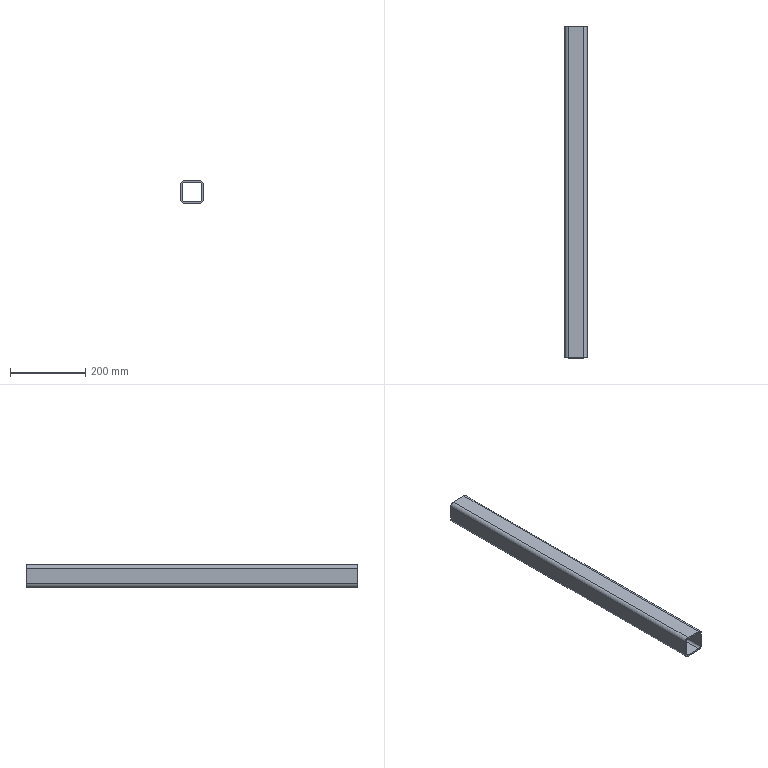Part | SolidWorks | features Extrusion 1 | 1 solid | 18 faces | box 60 x 880 x 60 mm | volume 740134 mm3 | plane 10 | cylinder 8 | commonest cylinder face diameters 12 x4 20 x4
STEP:
#1=CARTESIAN_POINT('',(20.,880.,30.));
#2=VERTEX_POINT('',#1);
#3=CARTESIAN_POINT('',(30.,880.,20.));
#4=VERTEX_POINT('',#3);
#5=CARTESIAN_POINT('',(20.,880.,20.));
#6=DIRECTION('',(0.,1.,0.));
#7=DIRECTION('',(0.,0.,1.));
#8=AXIS2_PLACEMENT_3D('',#5,#6,#7);
#9=CIRCLE('',#8,10.);
#10=EDGE_CURVE('',#2,#4,#9,.T.);
#11=ORIENTED_EDGE('',*,*,#10,.T.);
#12=CARTESIAN_POINT('',(30.,880.,-20.));
#13=VERTEX_POINT('',#12);
#14=CARTESIAN_POINT('',(30.,880.,20.));
#15=DIRECTION('',(0.,0.,-1.));
#16=VECTOR('',#15,1000.);
#17=LINE('',#14,#16);
#18=EDGE_CURVE('',#4,#13,#17,.T.);
#19=ORIENTED_EDGE('',*,*,#18,.T.);
#20=CARTESIAN_POINT('',(20.,880.,-30.));
#21=VERTEX_POINT('',#20);
#22=CARTESIAN_POINT('',(20.,880.,-20.));
#23=DIRECTION('',(0.,1.,0.));
#24=DIRECTION('',(0.,0.,-1.));
#25=AXIS2_PLACEMENT_3D('',#22,#23,#24);
#26=CIRCLE('',#25,10.);
#27=EDGE_CURVE('',#13,#21,#26,.T.);
#28=ORIENTED_EDGE('',*,*,#27,.T.);
#29=CARTESIAN_POINT('',(-20.,880.,-30.));
#30=VERTEX_POINT('',#29);
#31=CARTESIAN_POINT('',(-20.,880.,-30.));
#32=DIRECTION('',(-1.,0.,0.));
#33=VECTOR('',#32,1000.);
#34=LINE('',#31,#33);
#35=EDGE_CURVE('',#21,#30,#34,.T.);
#36=ORIENTED_EDGE('',*,*,#35,.T.);
#37=CARTESIAN_POINT('',(-30.,880.,-20.));
#38=VERTEX_POINT('',#37);
#39=CARTESIAN_POINT('',(-20.,880.,-20.));
#40=DIRECTION('',(0.,1.,0.));
#41=DIRECTION('',(0.,0.,-1.));
#42=AXIS2_PLACEMENT_3D('',#39,#40,#41);
#43=CIRCLE('',#42,10.);
#44=EDGE_CURVE('',#30,#38,#43,.T.);
#45=ORIENTED_EDGE('',*,*,#44,.T.);
#46=CARTESIAN_POINT('',(-30.,880.,20.));
#47=VERTEX_POINT('',#46);
#48=CARTESIAN_POINT('',(-30.,880.,20.));
#49=DIRECTION('',(0.,0.,1.));
#50=VECTOR('',#49,1000.);
#51=LINE('',#48,#50);
#52=EDGE_CURVE('',#38,#47,#51,.T.);
#53=ORIENTED_EDGE('',*,*,#52,.T.);
#54=CARTESIAN_POINT('',(-20.,880.,30.));
#55=VERTEX_POINT('',#54);
#56=CARTESIAN_POINT('',(-20.,880.,20.));
#57=DIRECTION('',(0.,1.,0.));
#58=DIRECTION('',(0.,0.,-1.));
#59=AXIS2_PLACEMENT_3D('',#56,#57,#58);
#60=CIRCLE('',#59,10.);
#61=EDGE_CURVE('',#47,#55,#60,.T.);
#62=ORIENTED_EDGE('',*,*,#61,.T.);
#63=CARTESIAN_POINT('',(-20.,880.,30.));
#64=DIRECTION('',(1.,0.,0.));
#65=VECTOR('',#64,1000.);
#66=LINE('',#63,#65);
#67=EDGE_CURVE('',#55,#2,#66,.T.);
#68=ORIENTED_EDGE('',*,*,#67,.T.);
#69=EDGE_LOOP('',(#11,#19,#28,#36,#45,#53,#62,#68));
#70=FACE_OUTER_BOUND('',#69,.T.);
#71=CARTESIAN_POINT('',(-20.,880.,26.));
#72=VERTEX_POINT('',#71);
#73=CARTESIAN_POINT('',(20.,880.,26.));
#74=VERTEX_POINT('',#73);
#75=CARTESIAN_POINT('',(-20.,880.,26.));
#76=DIRECTION('',(1.,0.,0.));
#77=VECTOR('',#76,1000.);
#78=LINE('',#75,#77);
#79=EDGE_CURVE('',#72,#74,#78,.T.);
#80=ORIENTED_EDGE('',*,*,#79,.F.);
#81=CARTESIAN_POINT('',(-26.,880.,20.));
#82=VERTEX_POINT('',#81);
#83=CARTESIAN_POINT('',(-20.,880.,20.));
#84=DIRECTION('',(0.,1.,0.));
#85=DIRECTION('',(0.,0.,-1.));
#86=AXIS2_PLACEMENT_3D('',#83,#84,#85);
#87=CIRCLE('',#86,6.);
#88=EDGE_CURVE('',#82,#72,#87,.T.);
#89=ORIENTED_EDGE('',*,*,#88,.F.);
#90=CARTESIAN_POINT('',(-26.,880.,-20.));
#91=VERTEX_POINT('',#90);
#92=CARTESIAN_POINT('',(-26.,880.,20.));
#93=DIRECTION('',(0.,0.,1.));
#94=VECTOR('',#93,1000.);
#95=LINE('',#92,#94);
#96=EDGE_CURVE('',#91,#82,#95,.T.);
#97=ORIENTED_EDGE('',*,*,#96,.F.);
#98=CARTESIAN_POINT('',(-20.,880.,-26.));
#99=VERTEX_POINT('',#98);
#100=CARTESIAN_POINT('',(-20.,880.,-20.));
#101=DIRECTION('',(0.,1.,0.));
#102=DIRECTION('',(0.,0.,-1.));
#103=AXIS2_PLACEMENT_3D('',#100,#101,#102);
#104=CIRCLE('',#103,6.);
#105=EDGE_CURVE('',#99,#91,#104,.T.);
#106=ORIENTED_EDGE('',*,*,#105,.F.);
#107=CARTESIAN_POINT('',(20.,880.,-26.));
#108=VERTEX_POINT('',#107);
#109=CARTESIAN_POINT('',(-20.,880.,-26.));
#110=DIRECTION('',(-1.,0.,0.));
#111=VECTOR('',#110,1000.);
#112=LINE('',#109,#111);
#113=EDGE_CURVE('',#108,#99,#112,.T.);
#114=ORIENTED_EDGE('',*,*,#113,.F.);
#115=CARTESIAN_POINT('',(26.,880.,-20.));
#116=VERTEX_POINT('',#115);
#117=CARTESIAN_POINT('',(20.,880.,-20.));
#118=DIRECTION('',(0.,1.,0.));
#119=DIRECTION('',(0.,0.,-1.));
#120=AXIS2_PLACEMENT_3D('',#117,#118,#119);
#121=CIRCLE('',#120,6.);
#122=EDGE_CURVE('',#116,#108,#121,.T.);
#123=ORIENTED_EDGE('',*,*,#122,.F.);
#124=CARTESIAN_POINT('',(26.,880.,20.));
#125=VERTEX_POINT('',#124);
#126=CARTESIAN_POINT('',(26.,880.,20.));
#127=DIRECTION('',(0.,0.,-1.));
#128=VECTOR('',#127,1000.);
#129=LINE('',#126,#128);
#130=EDGE_CURVE('',#125,#116,#129,.T.);
#131=ORIENTED_EDGE('',*,*,#130,.F.);
#132=CARTESIAN_POINT('',(20.,880.,20.));
#133=DIRECTION('',(0.,1.,0.));
#134=DIRECTION('',(0.,0.,1.));
#135=AXIS2_PLACEMENT_3D('',#132,#133,#134);
#136=CIRCLE('',#135,6.);
#137=EDGE_CURVE('',#74,#125,#136,.T.);
#138=ORIENTED_EDGE('',*,*,#137,.F.);
#139=EDGE_LOOP('',(#80,#89,#97,#106,#114,#123,#131,#138));
#140=FACE_BOUND('',#139,.T.);
#141=CARTESIAN_POINT('',(20.,880.,20.));
#142=DIRECTION('',(0.,1.,0.));
#143=DIRECTION('',(0.,0.,1.));
#144=AXIS2_PLACEMENT_3D('',#141,#142,#143);
#145=PLANE('',#144);
#146=ADVANCED_FACE('',(#70,#140),#145,.T.);
#147=CARTESIAN_POINT('',(20.,0.,30.));
#148=VERTEX_POINT('',#147);
#149=CARTESIAN_POINT('',(30.,0.,20.));
#150=VERTEX_POINT('',#149);
#151=CARTESIAN_POINT('',(20.,0.,20.));
#152=DIRECTION('',(0.,1.,0.));
#153=DIRECTION('',(0.,0.,1.));
#154=AXIS2_PLACEMENT_3D('',#151,#152,#153);
#155=CIRCLE('',#154,10.);
#156=EDGE_CURVE('',#148,#150,#155,.T.);
#157=ORIENTED_EDGE('',*,*,#156,.F.);
#158=CARTESIAN_POINT('',(-20.,0.,30.));
#159=VERTEX_POINT('',#158);
#160=CARTESIAN_POINT('',(-20.,0.,30.));
#161=DIRECTION('',(1.,0.,0.));
#162=VECTOR('',#161,1000.);
#163=LINE('',#160,#162);
#164=EDGE_CURVE('',#159,#148,#163,.T.);
#165=ORIENTED_EDGE('',*,*,#164,.F.);
#166=CARTESIAN_POINT('',(-30.,0.,20.));
#167=VERTEX_POINT('',#166);
#168=CARTESIAN_POINT('',(-20.,0.,20.));
#169=DIRECTION('',(0.,1.,0.));
#170=DIRECTION('',(0.,0.,-1.));
#171=AXIS2_PLACEMENT_3D('',#168,#169,#170);
#172=CIRCLE('',#171,10.);
#173=EDGE_CURVE('',#167,#159,#172,.T.);
#174=ORIENTED_EDGE('',*,*,#173,.F.);
#175=CARTESIAN_POINT('',(-30.,0.,-20.));
#176=VERTEX_POINT('',#175);
#177=CARTESIAN_POINT('',(-30.,0.,20.));
#178=DIRECTION('',(0.,0.,1.));
#179=VECTOR('',#178,1000.);
#180=LINE('',#177,#179);
#181=EDGE_CURVE('',#176,#167,#180,.T.);
#182=ORIENTED_EDGE('',*,*,#181,.F.);
#183=CARTESIAN_POINT('',(-20.,0.,-30.));
#184=VERTEX_POINT('',#183);
#185=CARTESIAN_POINT('',(-20.,0.,-20.));
#186=DIRECTION('',(0.,1.,0.));
#187=DIRECTION('',(0.,0.,-1.));
#188=AXIS2_PLACEMENT_3D('',#185,#186,#187);
#189=CIRCLE('',#188,10.);
#190=EDGE_CURVE('',#184,#176,#189,.T.);
#191=ORIENTED_EDGE('',*,*,#190,.F.);
#192=CARTESIAN_POINT('',(20.,0.,-30.));
#193=VERTEX_POINT('',#192);
#194=CARTESIAN_POINT('',(-20.,0.,-30.));
#195=DIRECTION('',(-1.,0.,0.));
#196=VECTOR('',#195,1000.);
#197=LINE('',#194,#196);
#198=EDGE_CURVE('',#193,#184,#197,.T.);
#199=ORIENTED_EDGE('',*,*,#198,.F.);
#200=CARTESIAN_POINT('',(30.,0.,-20.));
#201=VERTEX_POINT('',#200);
#202=CARTESIAN_POINT('',(20.,0.,-20.));
#203=DIRECTION('',(0.,1.,0.));
#204=DIRECTION('',(0.,0.,-1.));
#205=AXIS2_PLACEMENT_3D('',#202,#203,#204);
#206=CIRCLE('',#205,10.);
#207=EDGE_CURVE('',#201,#193,#206,.T.);
#208=ORIENTED_EDGE('',*,*,#207,.F.);
#209=CARTESIAN_POINT('',(30.,0.,20.));
#210=DIRECTION('',(0.,0.,-1.));
#211=VECTOR('',#210,1000.);
#212=LINE('',#209,#211);
#213=EDGE_CURVE('',#150,#201,#212,.T.);
#214=ORIENTED_EDGE('',*,*,#213,.F.);
#215=EDGE_LOOP('',(#157,#165,#174,#182,#191,#199,#208,#214));
#216=FACE_OUTER_BOUND('',#215,.T.);
#217=CARTESIAN_POINT('',(-26.,0.,20.));
#218=VERTEX_POINT('',#217);
#219=CARTESIAN_POINT('',(-20.,0.,26.));
#220=VERTEX_POINT('',#219);
#221=CARTESIAN_POINT('',(-20.,0.,20.));
#222=DIRECTION('',(0.,1.,0.));
#223=DIRECTION('',(0.,0.,-1.));
#224=AXIS2_PLACEMENT_3D('',#221,#222,#223);
#225=CIRCLE('',#224,6.);
#226=EDGE_CURVE('',#218,#220,#225,.T.);
#227=ORIENTED_EDGE('',*,*,#226,.T.);
#228=CARTESIAN_POINT('',(20.,0.,26.));
#229=VERTEX_POINT('',#228);
#230=CARTESIAN_POINT('',(-20.,0.,26.));
#231=DIRECTION('',(1.,0.,0.));
#232=VECTOR('',#231,1000.);
#233=LINE('',#230,#232);
#234=EDGE_CURVE('',#220,#229,#233,.T.);
#235=ORIENTED_EDGE('',*,*,#234,.T.);
#236=CARTESIAN_POINT('',(26.,0.,20.));
#237=VERTEX_POINT('',#236);
#238=CARTESIAN_POINT('',(20.,0.,20.));
#239=DIRECTION('',(0.,1.,0.));
#240=DIRECTION('',(0.,0.,1.));
#241=AXIS2_PLACEMENT_3D('',#238,#239,#240);
#242=CIRCLE('',#241,6.);
#243=EDGE_CURVE('',#229,#237,#242,.T.);
#244=ORIENTED_EDGE('',*,*,#243,.T.);
#245=CARTESIAN_POINT('',(26.,0.,-20.));
#246=VERTEX_POINT('',#245);
#247=CARTESIAN_POINT('',(26.,0.,20.));
#248=DIRECTION('',(0.,0.,-1.));
#249=VECTOR('',#248,1000.);
#250=LINE('',#247,#249);
#251=EDGE_CURVE('',#237,#246,#250,.T.);
#252=ORIENTED_EDGE('',*,*,#251,.T.);
#253=CARTESIAN_POINT('',(20.,0.,-26.));
#254=VERTEX_POINT('',#253);
#255=CARTESIAN_POINT('',(20.,0.,-20.));
#256=DIRECTION('',(0.,1.,0.));
#257=DIRECTION('',(0.,0.,-1.));
#258=AXIS2_PLACEMENT_3D('',#255,#256,#257);
#259=CIRCLE('',#258,6.);
#260=EDGE_CURVE('',#246,#254,#259,.T.);
#261=ORIENTED_EDGE('',*,*,#260,.T.);
#262=CARTESIAN_POINT('',(-20.,0.,-26.));
#263=VERTEX_POINT('',#262);
#264=CARTESIAN_POINT('',(-20.,0.,-26.));
#265=DIRECTION('',(-1.,0.,0.));
#266=VECTOR('',#265,1000.);
#267=LINE('',#264,#266);
#268=EDGE_CURVE('',#254,#263,#267,.T.);
#269=ORIENTED_EDGE('',*,*,#268,.T.);
#270=CARTESIAN_POINT('',(-26.,0.,-20.));
#271=VERTEX_POINT('',#270);
#272=CARTESIAN_POINT('',(-20.,0.,-20.));
#273=DIRECTION('',(0.,1.,0.));
#274=DIRECTION('',(0.,0.,-1.));
#275=AXIS2_PLACEMENT_3D('',#272,#273,#274);
#276=CIRCLE('',#275,6.);
#277=EDGE_CURVE('',#263,#271,#276,.T.);
#278=ORIENTED_EDGE('',*,*,#277,.T.);
#279=CARTESIAN_POINT('',(-26.,0.,20.));
#280=DIRECTION('',(0.,0.,1.));
#281=VECTOR('',#280,1000.);
#282=LINE('',#279,#281);
#283=EDGE_CURVE('',#271,#218,#282,.T.);
#284=ORIENTED_EDGE('',*,*,#283,.T.);
#285=EDGE_LOOP('',(#227,#235,#244,#252,#261,#269,#278,#284));
#286=FACE_BOUND('',#285,.T.);
#287=CARTESIAN_POINT('',(20.,0.,20.));
#288=DIRECTION('',(0.,1.,0.));
#289=DIRECTION('',(0.,0.,1.));
#290=AXIS2_PLACEMENT_3D('',#287,#288,#289);
#291=PLANE('',#290);
#292=ADVANCED_FACE('',(#216,#286),#291,.F.);
#293=ORIENTED_EDGE('',*,*,#156,.T.);
#294=CARTESIAN_POINT('',(30.,880.,20.));
#295=DIRECTION('',(0.,-1.,0.));
#296=VECTOR('',#295,1000.);
#297=LINE('',#294,#296);
#298=EDGE_CURVE('',#4,#150,#297,.T.);
#299=ORIENTED_EDGE('',*,*,#298,.F.);
#300=ORIENTED_EDGE('',*,*,#10,.F.);
#301=CARTESIAN_POINT('',(20.,880.,30.));
#302=DIRECTION('',(0.,-1.,0.));
#303=VECTOR('',#302,1000.);
#304=LINE('',#301,#303);
#305=EDGE_CURVE('',#2,#148,#304,.T.);
#306=ORIENTED_EDGE('',*,*,#305,.T.);
#307=EDGE_LOOP('',(#293,#299,#300,#306));
#308=FACE_OUTER_BOUND('',#307,.T.);
#309=CARTESIAN_POINT('',(20.,880.,20.));
#310=DIRECTION('',(0.,-1.,0.));
#311=DIRECTION('',(0.,0.,-1.));
#312=AXIS2_PLACEMENT_3D('',#309,#310,#311);
#313=CYLINDRICAL_SURFACE('',#312,10.);
#314=ADVANCED_FACE('',(#308),#313,.T.);
#315=ORIENTED_EDGE('',*,*,#213,.T.);
#316=CARTESIAN_POINT('',(30.,880.,-20.));
#317=DIRECTION('',(0.,-1.,0.));
#318=VECTOR('',#317,1000.);
#319=LINE('',#316,#318);
#320=EDGE_CURVE('',#13,#201,#319,.T.);
#321=ORIENTED_EDGE('',*,*,#320,.F.);
#322=ORIENTED_EDGE('',*,*,#18,.F.);
#323=ORIENTED_EDGE('',*,*,#298,.T.);
#324=EDGE_LOOP('',(#315,#321,#322,#323));
#325=FACE_OUTER_BOUND('',#324,.T.);
#326=CARTESIAN_POINT('',(30.,880.,20.));
#327=DIRECTION('',(-1.,0.,0.));
#328=DIRECTION('',(0.,0.,1.));
#329=AXIS2_PLACEMENT_3D('',#326,#327,#328);
#330=PLANE('',#329);
#331=ADVANCED_FACE('',(#325),#330,.F.);
#332=ORIENTED_EDGE('',*,*,#207,.T.);
#333=CARTESIAN_POINT('',(20.,880.,-30.));
#334=DIRECTION('',(0.,-1.,0.));
#335=VECTOR('',#334,1000.);
#336=LINE('',#333,#335);
#337=EDGE_CURVE('',#21,#193,#336,.T.);
#338=ORIENTED_EDGE('',*,*,#337,.F.);
#339=ORIENTED_EDGE('',*,*,#27,.F.);
#340=ORIENTED_EDGE('',*,*,#320,.T.);
#341=EDGE_LOOP('',(#332,#338,#339,#340));
#342=FACE_OUTER_BOUND('',#341,.T.);
#343=CARTESIAN_POINT('',(20.,880.,-20.));
#344=DIRECTION('',(0.,-1.,0.));
#345=DIRECTION('',(0.,0.,-1.));
#346=AXIS2_PLACEMENT_3D('',#343,#344,#345);
#347=CYLINDRICAL_SURFACE('',#346,10.);
#348=ADVANCED_FACE('',(#342),#347,.T.);
#349=ORIENTED_EDGE('',*,*,#198,.T.);
#350=CARTESIAN_POINT('',(-20.,880.,-30.));
#351=DIRECTION('',(0.,-1.,0.));
#352=VECTOR('',#351,1000.);
#353=LINE('',#350,#352);
#354=EDGE_CURVE('',#30,#184,#353,.T.);
#355=ORIENTED_EDGE('',*,*,#354,.F.);
#356=ORIENTED_EDGE('',*,*,#35,.F.);
#357=ORIENTED_EDGE('',*,*,#337,.T.);
#358=EDGE_LOOP('',(#349,#355,#356,#357));
#359=FACE_OUTER_BOUND('',#358,.T.);
#360=CARTESIAN_POINT('',(-20.,880.,-30.));
#361=DIRECTION('',(0.,0.,1.));
#362=DIRECTION('',(1.,0.,0.));
#363=AXIS2_PLACEMENT_3D('',#360,#361,#362);
#364=PLANE('',#363);
#365=ADVANCED_FACE('',(#359),#364,.F.);
#366=ORIENTED_EDGE('',*,*,#190,.T.);
#367=CARTESIAN_POINT('',(-30.,880.,-20.));
#368=DIRECTION('',(0.,-1.,0.));
#369=VECTOR('',#368,1000.);
#370=LINE('',#367,#369);
#371=EDGE_CURVE('',#38,#176,#370,.T.);
#372=ORIENTED_EDGE('',*,*,#371,.F.);
#373=ORIENTED_EDGE('',*,*,#44,.F.);
#374=ORIENTED_EDGE('',*,*,#354,.T.);
#375=EDGE_LOOP('',(#366,#372,#373,#374));
#376=FACE_OUTER_BOUND('',#375,.T.);
#377=CARTESIAN_POINT('',(-20.,880.,-20.));
#378=DIRECTION('',(0.,-1.,0.));
#379=DIRECTION('',(0.,0.,-1.));
#380=AXIS2_PLACEMENT_3D('',#377,#378,#379);
#381=CYLINDRICAL_SURFACE('',#380,10.);
#382=ADVANCED_FACE('',(#376),#381,.T.);
#383=ORIENTED_EDGE('',*,*,#181,.T.);
#384=CARTESIAN_POINT('',(-30.,880.,20.));
#385=DIRECTION('',(0.,-1.,0.));
#386=VECTOR('',#385,1000.);
#387=LINE('',#384,#386);
#388=EDGE_CURVE('',#47,#167,#387,.T.);
#389=ORIENTED_EDGE('',*,*,#388,.F.);
#390=ORIENTED_EDGE('',*,*,#52,.F.);
#391=ORIENTED_EDGE('',*,*,#371,.T.);
#392=EDGE_LOOP('',(#383,#389,#390,#391));
#393=FACE_OUTER_BOUND('',#392,.T.);
#394=CARTESIAN_POINT('',(-30.,880.,20.));
#395=DIRECTION('',(1.,0.,0.));
#396=DIRECTION('',(0.,0.,-1.));
#397=AXIS2_PLACEMENT_3D('',#394,#395,#396);
#398=PLANE('',#397);
#399=ADVANCED_FACE('',(#393),#398,.F.);
#400=ORIENTED_EDGE('',*,*,#173,.T.);
#401=CARTESIAN_POINT('',(-20.,880.,30.));
#402=DIRECTION('',(0.,-1.,0.));
#403=VECTOR('',#402,1000.);
#404=LINE('',#401,#403);
#405=EDGE_CURVE('',#55,#159,#404,.T.);
#406=ORIENTED_EDGE('',*,*,#405,.F.);
#407=ORIENTED_EDGE('',*,*,#61,.F.);
#408=ORIENTED_EDGE('',*,*,#388,.T.);
#409=EDGE_LOOP('',(#400,#406,#407,#408));
#410=FACE_OUTER_BOUND('',#409,.T.);
#411=CARTESIAN_POINT('',(-20.,880.,20.));
#412=DIRECTION('',(0.,-1.,0.));
#413=DIRECTION('',(0.,0.,-1.));
#414=AXIS2_PLACEMENT_3D('',#411,#412,#413);
#415=CYLINDRICAL_SURFACE('',#414,10.);
#416=ADVANCED_FACE('',(#410),#415,.T.);
#417=ORIENTED_EDGE('',*,*,#164,.T.);
#418=ORIENTED_EDGE('',*,*,#305,.F.);
#419=ORIENTED_EDGE('',*,*,#67,.F.);
#420=ORIENTED_EDGE('',*,*,#405,.T.);
#421=EDGE_LOOP('',(#417,#418,#419,#420));
#422=FACE_OUTER_BOUND('',#421,.T.);
#423=CARTESIAN_POINT('',(-20.,880.,30.));
#424=DIRECTION('',(0.,0.,-1.));
#425=DIRECTION('',(-1.,0.,0.));
#426=AXIS2_PLACEMENT_3D('',#423,#424,#425);
#427=PLANE('',#426);
#428=ADVANCED_FACE('',(#422),#427,.F.);
#429=ORIENTED_EDGE('',*,*,#226,.F.);
#430=CARTESIAN_POINT('',(-26.,880.,20.));
#431=DIRECTION('',(0.,-1.,0.));
#432=VECTOR('',#431,1000.);
#433=LINE('',#430,#432);
#434=EDGE_CURVE('',#82,#218,#433,.T.);
#435=ORIENTED_EDGE('',*,*,#434,.F.);
#436=ORIENTED_EDGE('',*,*,#88,.T.);
#437=CARTESIAN_POINT('',(-20.,880.,26.));
#438=DIRECTION('',(0.,-1.,0.));
#439=VECTOR('',#438,1000.);
#440=LINE('',#437,#439);
#441=EDGE_CURVE('',#72,#220,#440,.T.);
#442=ORIENTED_EDGE('',*,*,#441,.T.);
#443=EDGE_LOOP('',(#429,#435,#436,#442));
#444=FACE_OUTER_BOUND('',#443,.T.);
#445=CARTESIAN_POINT('',(-20.,880.,20.));
#446=DIRECTION('',(0.,-1.,0.));
#447=DIRECTION('',(0.,0.,-1.));
#448=AXIS2_PLACEMENT_3D('',#445,#446,#447);
#449=CYLINDRICAL_SURFACE('',#448,6.);
#450=ADVANCED_FACE('',(#444),#449,.F.);
#451=ORIENTED_EDGE('',*,*,#234,.F.);
#452=ORIENTED_EDGE('',*,*,#441,.F.);
#453=ORIENTED_EDGE('',*,*,#79,.T.);
#454=CARTESIAN_POINT('',(20.,880.,26.));
#455=DIRECTION('',(0.,-1.,0.));
#456=VECTOR('',#455,1000.);
#457=LINE('',#454,#456);
#458=EDGE_CURVE('',#74,#229,#457,.T.);
#459=ORIENTED_EDGE('',*,*,#458,.T.);
#460=EDGE_LOOP('',(#451,#452,#453,#459));
#461=FACE_OUTER_BOUND('',#460,.T.);
#462=CARTESIAN_POINT('',(-20.,880.,26.));
#463=DIRECTION('',(0.,0.,-1.));
#464=DIRECTION('',(-1.,0.,0.));
#465=AXIS2_PLACEMENT_3D('',#462,#463,#464);
#466=PLANE('',#465);
#467=ADVANCED_FACE('',(#461),#466,.T.);
#468=ORIENTED_EDGE('',*,*,#243,.F.);
#469=ORIENTED_EDGE('',*,*,#458,.F.);
#470=ORIENTED_EDGE('',*,*,#137,.T.);
#471=CARTESIAN_POINT('',(26.,880.,20.));
#472=DIRECTION('',(0.,-1.,0.));
#473=VECTOR('',#472,1000.);
#474=LINE('',#471,#473);
#475=EDGE_CURVE('',#125,#237,#474,.T.);
#476=ORIENTED_EDGE('',*,*,#475,.T.);
#477=EDGE_LOOP('',(#468,#469,#470,#476));
#478=FACE_OUTER_BOUND('',#477,.T.);
#479=CARTESIAN_POINT('',(20.,880.,20.));
#480=DIRECTION('',(0.,-1.,0.));
#481=DIRECTION('',(0.,0.,-1.));
#482=AXIS2_PLACEMENT_3D('',#479,#480,#481);
#483=CYLINDRICAL_SURFACE('',#482,6.);
#484=ADVANCED_FACE('',(#478),#483,.F.);
#485=ORIENTED_EDGE('',*,*,#251,.F.);
#486=ORIENTED_EDGE('',*,*,#475,.F.);
#487=ORIENTED_EDGE('',*,*,#130,.T.);
#488=CARTESIAN_POINT('',(26.,880.,-20.));
#489=DIRECTION('',(0.,-1.,0.));
#490=VECTOR('',#489,1000.);
#491=LINE('',#488,#490);
#492=EDGE_CURVE('',#116,#246,#491,.T.);
#493=ORIENTED_EDGE('',*,*,#492,.T.);
#494=EDGE_LOOP('',(#485,#486,#487,#493));
#495=FACE_OUTER_BOUND('',#494,.T.);
#496=CARTESIAN_POINT('',(26.,880.,20.));
#497=DIRECTION('',(-1.,0.,0.));
#498=DIRECTION('',(0.,0.,1.));
#499=AXIS2_PLACEMENT_3D('',#496,#497,#498);
#500=PLANE('',#499);
#501=ADVANCED_FACE('',(#495),#500,.T.);
#502=ORIENTED_EDGE('',*,*,#260,.F.);
#503=ORIENTED_EDGE('',*,*,#492,.F.);
#504=ORIENTED_EDGE('',*,*,#122,.T.);
#505=CARTESIAN_POINT('',(20.,880.,-26.));
#506=DIRECTION('',(0.,-1.,0.));
#507=VECTOR('',#506,1000.);
#508=LINE('',#505,#507);
#509=EDGE_CURVE('',#108,#254,#508,.T.);
#510=ORIENTED_EDGE('',*,*,#509,.T.);
#511=EDGE_LOOP('',(#502,#503,#504,#510));
#512=FACE_OUTER_BOUND('',#511,.T.);
#513=CARTESIAN_POINT('',(20.,880.,-20.));
#514=DIRECTION('',(0.,-1.,0.));
#515=DIRECTION('',(0.,0.,-1.));
#516=AXIS2_PLACEMENT_3D('',#513,#514,#515);
#517=CYLINDRICAL_SURFACE('',#516,6.);
#518=ADVANCED_FACE('',(#512),#517,.F.);
#519=ORIENTED_EDGE('',*,*,#268,.F.);
#520=ORIENTED_EDGE('',*,*,#509,.F.);
#521=ORIENTED_EDGE('',*,*,#113,.T.);
#522=CARTESIAN_POINT('',(-20.,880.,-26.));
#523=DIRECTION('',(0.,-1.,0.));
#524=VECTOR('',#523,1000.);
#525=LINE('',#522,#524);
#526=EDGE_CURVE('',#99,#263,#525,.T.);
#527=ORIENTED_EDGE('',*,*,#526,.T.);
#528=EDGE_LOOP('',(#519,#520,#521,#527));
#529=FACE_OUTER_BOUND('',#528,.T.);
#530=CARTESIAN_POINT('',(-20.,880.,-26.));
#531=DIRECTION('',(0.,0.,1.));
#532=DIRECTION('',(1.,0.,0.));
#533=AXIS2_PLACEMENT_3D('',#530,#531,#532);
#534=PLANE('',#533);
#535=ADVANCED_FACE('',(#529),#534,.T.);
#536=ORIENTED_EDGE('',*,*,#277,.F.);
#537=ORIENTED_EDGE('',*,*,#526,.F.);
#538=ORIENTED_EDGE('',*,*,#105,.T.);
#539=CARTESIAN_POINT('',(-26.,880.,-20.));
#540=DIRECTION('',(0.,-1.,0.));
#541=VECTOR('',#540,1000.);
#542=LINE('',#539,#541);
#543=EDGE_CURVE('',#91,#271,#542,.T.);
#544=ORIENTED_EDGE('',*,*,#543,.T.);
#545=EDGE_LOOP('',(#536,#537,#538,#544));
#546=FACE_OUTER_BOUND('',#545,.T.);
#547=CARTESIAN_POINT('',(-20.,880.,-20.));
#548=DIRECTION('',(0.,-1.,0.));
#549=DIRECTION('',(0.,0.,-1.));
#550=AXIS2_PLACEMENT_3D('',#547,#548,#549);
#551=CYLINDRICAL_SURFACE('',#550,6.);
#552=ADVANCED_FACE('',(#546),#551,.F.);
#553=ORIENTED_EDGE('',*,*,#283,.F.);
#554=ORIENTED_EDGE('',*,*,#543,.F.);
#555=ORIENTED_EDGE('',*,*,#96,.T.);
#556=ORIENTED_EDGE('',*,*,#434,.T.);
#557=EDGE_LOOP('',(#553,#554,#555,#556));
#558=FACE_OUTER_BOUND('',#557,.T.);
#559=CARTESIAN_POINT('',(-26.,880.,20.));
#560=DIRECTION('',(1.,0.,0.));
#561=DIRECTION('',(0.,0.,-1.));
#562=AXIS2_PLACEMENT_3D('',#559,#560,#561);
#563=PLANE('',#562);
#564=ADVANCED_FACE('',(#558),#563,.T.);
#565=CLOSED_SHELL('',(#146,#292,#314,#331,#348,#365,#382,#399,#416,#428,#450,#467,#484,#501,#518,#535,#552,#564));
#566=MANIFOLD_SOLID_BREP('',#565);
#567=CARTESIAN_POINT('',(0.,0.,0.));
#568=DIRECTION('',(0.,0.,1.));
#569=DIRECTION('',(1.,0.,0.));
#570=AXIS2_PLACEMENT_3D('',#567,#568,#569);
#571=(LENGTH_UNIT()NAMED_UNIT(*)SI_UNIT(.MILLI.,.METRE.));
#572=UNCERTAINTY_MEASURE_WITH_UNIT(LENGTH_MEASURE(0.00001),#571,'','');
#573=(NAMED_UNIT(*)PLANE_ANGLE_UNIT()SI_UNIT($,.RADIAN.));
#574=(NAMED_UNIT(*)SI_UNIT($,.STERADIAN.)SOLID_ANGLE_UNIT());
#575=(GEOMETRIC_REPRESENTATION_CONTEXT(3)GLOBAL_UNCERTAINTY_ASSIGNED_CONTEXT((#572))GLOBAL_UNIT_ASSIGNED_CONTEXT((#571,#573,#574))REPRESENTATION_CONTEXT('',''));
#576=ADVANCED_BREP_SHAPE_REPRESENTATION('',(#566,#570),#575);